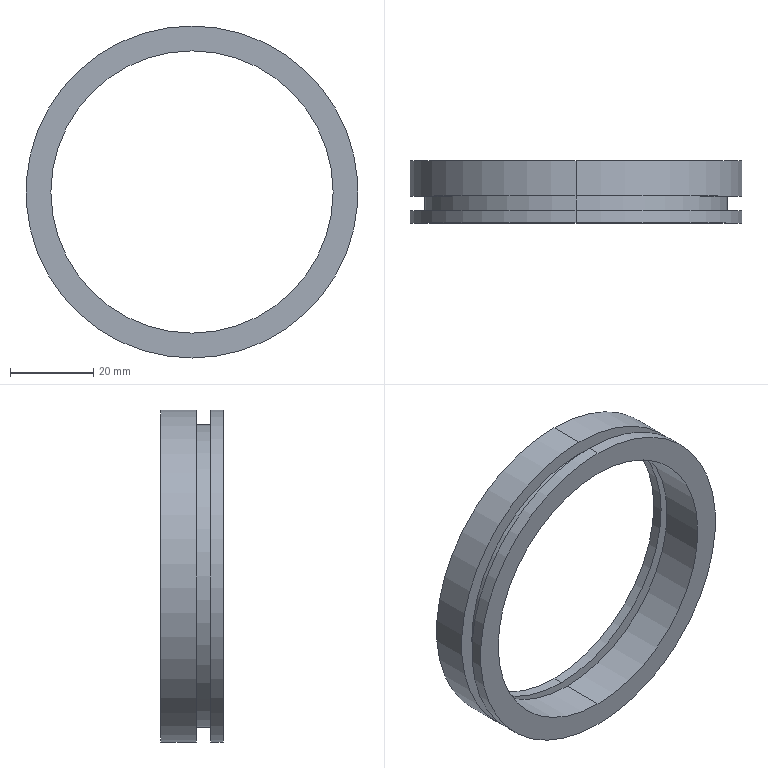Part | SolidWorks | features Revolution 1 | 1 solid | 18 faces | box 80 x 15 x 80 mm | volume 16407 mm3 | cylinder 12 | plane 6 | commonest cylinder face diameters 68 x4 80 x4 73 x2 75 x2
STEP:
#1=CARTESIAN_POINT('',(34.,12.5,37.5));
#2=VERTEX_POINT('',#1);
#3=CARTESIAN_POINT('',(34.,12.5,-37.5));
#4=VERTEX_POINT('',#3);
#5=CARTESIAN_POINT('',(34.,12.5,0.));
#6=DIRECTION('',(0.,-1.,0.));
#7=DIRECTION('',(0.,0.,-1.));
#8=AXIS2_PLACEMENT_3D('',#5,#6,#7);
#9=CIRCLE('',#8,37.5);
#10=EDGE_CURVE('',#2,#4,#9,.T.);
#11=ORIENTED_EDGE('',*,*,#10,.F.);
#12=CARTESIAN_POINT('',(34.,10.5,37.5));
#13=VERTEX_POINT('',#12);
#14=CARTESIAN_POINT('',(34.,0.,37.5));
#15=DIRECTION('',(0.,-1.,0.));
#16=VECTOR('',#15,1000.);
#17=LINE('',#14,#16);
#18=EDGE_CURVE('',#2,#13,#17,.T.);
#19=ORIENTED_EDGE('',*,*,#18,.T.);
#20=CARTESIAN_POINT('',(34.,10.5,-37.5));
#21=VERTEX_POINT('',#20);
#22=CARTESIAN_POINT('',(34.,10.5,0.));
#23=DIRECTION('',(0.,-1.,0.));
#24=DIRECTION('',(0.,0.,-1.));
#25=AXIS2_PLACEMENT_3D('',#22,#23,#24);
#26=CIRCLE('',#25,37.5);
#27=EDGE_CURVE('',#13,#21,#26,.T.);
#28=ORIENTED_EDGE('',*,*,#27,.T.);
#29=CARTESIAN_POINT('',(34.,0.,-37.5));
#30=DIRECTION('',(0.,-1.,0.));
#31=VECTOR('',#30,1000.);
#32=LINE('',#29,#31);
#33=EDGE_CURVE('',#4,#21,#32,.T.);
#34=ORIENTED_EDGE('',*,*,#33,.F.);
#35=EDGE_LOOP('',(#11,#19,#28,#34));
#36=FACE_OUTER_BOUND('',#35,.T.);
#37=CARTESIAN_POINT('',(34.,0.,0.));
#38=DIRECTION('',(0.,-1.,0.));
#39=DIRECTION('',(0.,0.,-1.));
#40=AXIS2_PLACEMENT_3D('',#37,#38,#39);
#41=CYLINDRICAL_SURFACE('',#40,37.5);
#42=ADVANCED_FACE('',(#36),#41,.F.);
#43=CARTESIAN_POINT('',(34.,15.,34.));
#44=VERTEX_POINT('',#43);
#45=CARTESIAN_POINT('',(34.,15.,-34.));
#46=VERTEX_POINT('',#45);
#47=CARTESIAN_POINT('',(34.,15.,0.));
#48=DIRECTION('',(0.,-1.,0.));
#49=DIRECTION('',(0.,0.,-1.));
#50=AXIS2_PLACEMENT_3D('',#47,#48,#49);
#51=CIRCLE('',#50,34.);
#52=EDGE_CURVE('',#44,#46,#51,.T.);
#53=ORIENTED_EDGE('',*,*,#52,.F.);
#54=CARTESIAN_POINT('',(34.,12.5,34.));
#55=VERTEX_POINT('',#54);
#56=CARTESIAN_POINT('',(34.,0.,34.));
#57=DIRECTION('',(0.,-1.,0.));
#58=VECTOR('',#57,1000.);
#59=LINE('',#56,#58);
#60=EDGE_CURVE('',#44,#55,#59,.T.);
#61=ORIENTED_EDGE('',*,*,#60,.T.);
#62=CARTESIAN_POINT('',(34.,12.5,-34.));
#63=VERTEX_POINT('',#62);
#64=CARTESIAN_POINT('',(34.,12.5,0.));
#65=DIRECTION('',(0.,-1.,0.));
#66=DIRECTION('',(0.,0.,-1.));
#67=AXIS2_PLACEMENT_3D('',#64,#65,#66);
#68=CIRCLE('',#67,34.);
#69=EDGE_CURVE('',#55,#63,#68,.T.);
#70=ORIENTED_EDGE('',*,*,#69,.T.);
#71=CARTESIAN_POINT('',(34.,0.,-34.));
#72=DIRECTION('',(0.,-1.,0.));
#73=VECTOR('',#72,1000.);
#74=LINE('',#71,#73);
#75=EDGE_CURVE('',#46,#63,#74,.T.);
#76=ORIENTED_EDGE('',*,*,#75,.F.);
#77=EDGE_LOOP('',(#53,#61,#70,#76));
#78=FACE_OUTER_BOUND('',#77,.T.);
#79=CARTESIAN_POINT('',(34.,0.,0.));
#80=DIRECTION('',(0.,-1.,0.));
#81=DIRECTION('',(0.,0.,-1.));
#82=AXIS2_PLACEMENT_3D('',#79,#80,#81);
#83=CYLINDRICAL_SURFACE('',#82,34.);
#84=ADVANCED_FACE('',(#78),#83,.F.);
#85=CARTESIAN_POINT('',(34.,15.,-40.));
#86=VERTEX_POINT('',#85);
#87=CARTESIAN_POINT('',(34.,15.,40.));
#88=VERTEX_POINT('',#87);
#89=CARTESIAN_POINT('',(34.,15.,0.));
#90=DIRECTION('',(0.,-1.,0.));
#91=DIRECTION('',(0.,0.,-1.));
#92=AXIS2_PLACEMENT_3D('',#89,#90,#91);
#93=CIRCLE('',#92,40.);
#94=EDGE_CURVE('',#86,#88,#93,.T.);
#95=ORIENTED_EDGE('',*,*,#94,.T.);
#96=CARTESIAN_POINT('',(34.,6.5,40.));
#97=VERTEX_POINT('',#96);
#98=CARTESIAN_POINT('',(34.,0.,40.));
#99=DIRECTION('',(0.,-1.,0.));
#100=VECTOR('',#99,1000.);
#101=LINE('',#98,#100);
#102=EDGE_CURVE('',#88,#97,#101,.T.);
#103=ORIENTED_EDGE('',*,*,#102,.T.);
#104=CARTESIAN_POINT('',(34.,6.5,-40.));
#105=VERTEX_POINT('',#104);
#106=CARTESIAN_POINT('',(34.,6.5,0.));
#107=DIRECTION('',(0.,-1.,0.));
#108=DIRECTION('',(0.,0.,-1.));
#109=AXIS2_PLACEMENT_3D('',#106,#107,#108);
#110=CIRCLE('',#109,40.);
#111=EDGE_CURVE('',#105,#97,#110,.T.);
#112=ORIENTED_EDGE('',*,*,#111,.F.);
#113=CARTESIAN_POINT('',(34.,0.,-40.));
#114=DIRECTION('',(0.,-1.,0.));
#115=VECTOR('',#114,1000.);
#116=LINE('',#113,#115);
#117=EDGE_CURVE('',#86,#105,#116,.T.);
#118=ORIENTED_EDGE('',*,*,#117,.F.);
#119=EDGE_LOOP('',(#95,#103,#112,#118));
#120=FACE_OUTER_BOUND('',#119,.T.);
#121=CARTESIAN_POINT('',(34.,0.,0.));
#122=DIRECTION('',(0.,-1.,0.));
#123=DIRECTION('',(0.,0.,-1.));
#124=AXIS2_PLACEMENT_3D('',#121,#122,#123);
#125=CYLINDRICAL_SURFACE('',#124,40.);
#126=ADVANCED_FACE('',(#120),#125,.T.);
#127=CARTESIAN_POINT('',(34.,6.5,-36.5));
#128=VERTEX_POINT('',#127);
#129=CARTESIAN_POINT('',(34.,6.5,36.5));
#130=VERTEX_POINT('',#129);
#131=CARTESIAN_POINT('',(34.,6.5,0.));
#132=DIRECTION('',(0.,-1.,0.));
#133=DIRECTION('',(0.,0.,-1.));
#134=AXIS2_PLACEMENT_3D('',#131,#132,#133);
#135=CIRCLE('',#134,36.5);
#136=EDGE_CURVE('',#128,#130,#135,.T.);
#137=ORIENTED_EDGE('',*,*,#136,.T.);
#138=CARTESIAN_POINT('',(34.,3.,36.5));
#139=VERTEX_POINT('',#138);
#140=CARTESIAN_POINT('',(34.,0.,36.5));
#141=DIRECTION('',(0.,-1.,0.));
#142=VECTOR('',#141,1000.);
#143=LINE('',#140,#142);
#144=EDGE_CURVE('',#130,#139,#143,.T.);
#145=ORIENTED_EDGE('',*,*,#144,.T.);
#146=CARTESIAN_POINT('',(34.,3.,-36.5));
#147=VERTEX_POINT('',#146);
#148=CARTESIAN_POINT('',(34.,3.,0.));
#149=DIRECTION('',(0.,-1.,0.));
#150=DIRECTION('',(0.,0.,-1.));
#151=AXIS2_PLACEMENT_3D('',#148,#149,#150);
#152=CIRCLE('',#151,36.5);
#153=EDGE_CURVE('',#147,#139,#152,.T.);
#154=ORIENTED_EDGE('',*,*,#153,.F.);
#155=CARTESIAN_POINT('',(34.,0.,-36.5));
#156=DIRECTION('',(0.,-1.,0.));
#157=VECTOR('',#156,1000.);
#158=LINE('',#155,#157);
#159=EDGE_CURVE('',#128,#147,#158,.T.);
#160=ORIENTED_EDGE('',*,*,#159,.F.);
#161=EDGE_LOOP('',(#137,#145,#154,#160));
#162=FACE_OUTER_BOUND('',#161,.T.);
#163=CARTESIAN_POINT('',(34.,0.,0.));
#164=DIRECTION('',(0.,-1.,0.));
#165=DIRECTION('',(0.,0.,-1.));
#166=AXIS2_PLACEMENT_3D('',#163,#164,#165);
#167=CYLINDRICAL_SURFACE('',#166,36.5);
#168=ADVANCED_FACE('',(#162),#167,.T.);
#169=CARTESIAN_POINT('',(34.,3.,-40.));
#170=VERTEX_POINT('',#169);
#171=CARTESIAN_POINT('',(34.,3.,40.));
#172=VERTEX_POINT('',#171);
#173=CARTESIAN_POINT('',(34.,3.,0.));
#174=DIRECTION('',(0.,-1.,0.));
#175=DIRECTION('',(0.,0.,-1.));
#176=AXIS2_PLACEMENT_3D('',#173,#174,#175);
#177=CIRCLE('',#176,40.);
#178=EDGE_CURVE('',#170,#172,#177,.T.);
#179=ORIENTED_EDGE('',*,*,#178,.T.);
#180=CARTESIAN_POINT('',(34.,0.,40.));
#181=VERTEX_POINT('',#180);
#182=CARTESIAN_POINT('',(34.,0.,40.));
#183=DIRECTION('',(0.,-1.,0.));
#184=VECTOR('',#183,1000.);
#185=LINE('',#182,#184);
#186=EDGE_CURVE('',#172,#181,#185,.T.);
#187=ORIENTED_EDGE('',*,*,#186,.T.);
#188=CARTESIAN_POINT('',(34.,0.,-40.));
#189=VERTEX_POINT('',#188);
#190=CARTESIAN_POINT('',(34.,0.,0.));
#191=DIRECTION('',(0.,-1.,0.));
#192=DIRECTION('',(0.,0.,-1.));
#193=AXIS2_PLACEMENT_3D('',#190,#191,#192);
#194=CIRCLE('',#193,40.);
#195=EDGE_CURVE('',#189,#181,#194,.T.);
#196=ORIENTED_EDGE('',*,*,#195,.F.);
#197=CARTESIAN_POINT('',(34.,0.,-40.));
#198=DIRECTION('',(0.,-1.,0.));
#199=VECTOR('',#198,1000.);
#200=LINE('',#197,#199);
#201=EDGE_CURVE('',#170,#189,#200,.T.);
#202=ORIENTED_EDGE('',*,*,#201,.F.);
#203=EDGE_LOOP('',(#179,#187,#196,#202));
#204=FACE_OUTER_BOUND('',#203,.T.);
#205=CARTESIAN_POINT('',(34.,0.,0.));
#206=DIRECTION('',(0.,-1.,0.));
#207=DIRECTION('',(0.,0.,-1.));
#208=AXIS2_PLACEMENT_3D('',#205,#206,#207);
#209=CYLINDRICAL_SURFACE('',#208,40.);
#210=ADVANCED_FACE('',(#204),#209,.T.);
#211=CARTESIAN_POINT('',(34.,10.5,34.));
#212=VERTEX_POINT('',#211);
#213=CARTESIAN_POINT('',(34.,10.5,-34.));
#214=VERTEX_POINT('',#213);
#215=CARTESIAN_POINT('',(34.,10.5,0.));
#216=DIRECTION('',(0.,-1.,0.));
#217=DIRECTION('',(0.,0.,-1.));
#218=AXIS2_PLACEMENT_3D('',#215,#216,#217);
#219=CIRCLE('',#218,34.);
#220=EDGE_CURVE('',#212,#214,#219,.T.);
#221=ORIENTED_EDGE('',*,*,#220,.F.);
#222=CARTESIAN_POINT('',(34.,0.,34.));
#223=VERTEX_POINT('',#222);
#224=CARTESIAN_POINT('',(34.,0.,34.));
#225=DIRECTION('',(0.,-1.,0.));
#226=VECTOR('',#225,1000.);
#227=LINE('',#224,#226);
#228=EDGE_CURVE('',#212,#223,#227,.T.);
#229=ORIENTED_EDGE('',*,*,#228,.T.);
#230=CARTESIAN_POINT('',(34.,0.,-34.));
#231=VERTEX_POINT('',#230);
#232=CARTESIAN_POINT('',(34.,0.,0.));
#233=DIRECTION('',(0.,-1.,0.));
#234=DIRECTION('',(0.,0.,-1.));
#235=AXIS2_PLACEMENT_3D('',#232,#233,#234);
#236=CIRCLE('',#235,34.);
#237=EDGE_CURVE('',#223,#231,#236,.T.);
#238=ORIENTED_EDGE('',*,*,#237,.T.);
#239=CARTESIAN_POINT('',(34.,0.,-34.));
#240=DIRECTION('',(0.,-1.,0.));
#241=VECTOR('',#240,1000.);
#242=LINE('',#239,#241);
#243=EDGE_CURVE('',#214,#231,#242,.T.);
#244=ORIENTED_EDGE('',*,*,#243,.F.);
#245=EDGE_LOOP('',(#221,#229,#238,#244));
#246=FACE_OUTER_BOUND('',#245,.T.);
#247=CARTESIAN_POINT('',(34.,0.,0.));
#248=DIRECTION('',(0.,-1.,0.));
#249=DIRECTION('',(0.,0.,-1.));
#250=AXIS2_PLACEMENT_3D('',#247,#248,#249);
#251=CYLINDRICAL_SURFACE('',#250,34.);
#252=ADVANCED_FACE('',(#246),#251,.F.);
#253=ORIENTED_EDGE('',*,*,#228,.F.);
#254=CARTESIAN_POINT('',(34.,10.5,0.));
#255=DIRECTION('',(0.,-1.,0.));
#256=DIRECTION('',(0.,0.,-1.));
#257=AXIS2_PLACEMENT_3D('',#254,#255,#256);
#258=CIRCLE('',#257,34.);
#259=EDGE_CURVE('',#214,#212,#258,.T.);
#260=ORIENTED_EDGE('',*,*,#259,.F.);
#261=ORIENTED_EDGE('',*,*,#243,.T.);
#262=CARTESIAN_POINT('',(34.,0.,0.));
#263=DIRECTION('',(0.,-1.,0.));
#264=DIRECTION('',(0.,0.,-1.));
#265=AXIS2_PLACEMENT_3D('',#262,#263,#264);
#266=CIRCLE('',#265,34.);
#267=EDGE_CURVE('',#231,#223,#266,.T.);
#268=ORIENTED_EDGE('',*,*,#267,.T.);
#269=EDGE_LOOP('',(#253,#260,#261,#268));
#270=FACE_OUTER_BOUND('',#269,.T.);
#271=CARTESIAN_POINT('',(34.,0.,0.));
#272=DIRECTION('',(0.,-1.,0.));
#273=DIRECTION('',(0.,0.,-1.));
#274=AXIS2_PLACEMENT_3D('',#271,#272,#273);
#275=CYLINDRICAL_SURFACE('',#274,34.);
#276=ADVANCED_FACE('',(#270),#275,.F.);
#277=ORIENTED_EDGE('',*,*,#267,.F.);
#278=ORIENTED_EDGE('',*,*,#237,.F.);
#279=EDGE_LOOP('',(#277,#278));
#280=FACE_BOUND('',#279,.T.);
#281=ORIENTED_EDGE('',*,*,#195,.T.);
#282=CARTESIAN_POINT('',(34.,0.,0.));
#283=DIRECTION('',(0.,-1.,0.));
#284=DIRECTION('',(0.,0.,-1.));
#285=AXIS2_PLACEMENT_3D('',#282,#283,#284);
#286=CIRCLE('',#285,40.);
#287=EDGE_CURVE('',#181,#189,#286,.T.);
#288=ORIENTED_EDGE('',*,*,#287,.T.);
#289=EDGE_LOOP('',(#281,#288));
#290=FACE_OUTER_BOUND('',#289,.T.);
#291=CARTESIAN_POINT('',(0.,0.,0.));
#292=DIRECTION('',(0.,1.,0.));
#293=DIRECTION('',(0.,0.,1.));
#294=AXIS2_PLACEMENT_3D('',#291,#292,#293);
#295=PLANE('',#294);
#296=ADVANCED_FACE('',(#280,#290),#295,.F.);
#297=ORIENTED_EDGE('',*,*,#186,.F.);
#298=CARTESIAN_POINT('',(34.,3.,0.));
#299=DIRECTION('',(0.,-1.,0.));
#300=DIRECTION('',(0.,0.,-1.));
#301=AXIS2_PLACEMENT_3D('',#298,#299,#300);
#302=CIRCLE('',#301,40.);
#303=EDGE_CURVE('',#172,#170,#302,.T.);
#304=ORIENTED_EDGE('',*,*,#303,.T.);
#305=ORIENTED_EDGE('',*,*,#201,.T.);
#306=ORIENTED_EDGE('',*,*,#287,.F.);
#307=EDGE_LOOP('',(#297,#304,#305,#306));
#308=FACE_OUTER_BOUND('',#307,.T.);
#309=CARTESIAN_POINT('',(34.,0.,0.));
#310=DIRECTION('',(0.,-1.,0.));
#311=DIRECTION('',(0.,0.,-1.));
#312=AXIS2_PLACEMENT_3D('',#309,#310,#311);
#313=CYLINDRICAL_SURFACE('',#312,40.);
#314=ADVANCED_FACE('',(#308),#313,.T.);
#315=ORIENTED_EDGE('',*,*,#178,.F.);
#316=ORIENTED_EDGE('',*,*,#303,.F.);
#317=EDGE_LOOP('',(#315,#316));
#318=FACE_OUTER_BOUND('',#317,.T.);
#319=ORIENTED_EDGE('',*,*,#153,.T.);
#320=CARTESIAN_POINT('',(34.,3.,0.));
#321=DIRECTION('',(0.,-1.,0.));
#322=DIRECTION('',(0.,0.,-1.));
#323=AXIS2_PLACEMENT_3D('',#320,#321,#322);
#324=CIRCLE('',#323,36.5);
#325=EDGE_CURVE('',#139,#147,#324,.T.);
#326=ORIENTED_EDGE('',*,*,#325,.T.);
#327=EDGE_LOOP('',(#319,#326));
#328=FACE_BOUND('',#327,.T.);
#329=CARTESIAN_POINT('',(-2.5,3.,0.));
#330=DIRECTION('',(0.,-1.,0.));
#331=DIRECTION('',(0.,0.,-1.));
#332=AXIS2_PLACEMENT_3D('',#329,#330,#331);
#333=PLANE('',#332);
#334=ADVANCED_FACE('',(#318,#328),#333,.F.);
#335=ORIENTED_EDGE('',*,*,#144,.F.);
#336=CARTESIAN_POINT('',(34.,6.5,0.));
#337=DIRECTION('',(0.,-1.,0.));
#338=DIRECTION('',(0.,0.,-1.));
#339=AXIS2_PLACEMENT_3D('',#336,#337,#338);
#340=CIRCLE('',#339,36.5);
#341=EDGE_CURVE('',#130,#128,#340,.T.);
#342=ORIENTED_EDGE('',*,*,#341,.T.);
#343=ORIENTED_EDGE('',*,*,#159,.T.);
#344=ORIENTED_EDGE('',*,*,#325,.F.);
#345=EDGE_LOOP('',(#335,#342,#343,#344));
#346=FACE_OUTER_BOUND('',#345,.T.);
#347=CARTESIAN_POINT('',(34.,0.,0.));
#348=DIRECTION('',(0.,-1.,0.));
#349=DIRECTION('',(0.,0.,-1.));
#350=AXIS2_PLACEMENT_3D('',#347,#348,#349);
#351=CYLINDRICAL_SURFACE('',#350,36.5);
#352=ADVANCED_FACE('',(#346),#351,.T.);
#353=ORIENTED_EDGE('',*,*,#136,.F.);
#354=ORIENTED_EDGE('',*,*,#341,.F.);
#355=EDGE_LOOP('',(#353,#354));
#356=FACE_BOUND('',#355,.T.);
#357=ORIENTED_EDGE('',*,*,#111,.T.);
#358=CARTESIAN_POINT('',(34.,6.5,0.));
#359=DIRECTION('',(0.,-1.,0.));
#360=DIRECTION('',(0.,0.,-1.));
#361=AXIS2_PLACEMENT_3D('',#358,#359,#360);
#362=CIRCLE('',#361,40.);
#363=EDGE_CURVE('',#97,#105,#362,.T.);
#364=ORIENTED_EDGE('',*,*,#363,.T.);
#365=EDGE_LOOP('',(#357,#364));
#366=FACE_OUTER_BOUND('',#365,.T.);
#367=CARTESIAN_POINT('',(-6.,6.5,0.));
#368=DIRECTION('',(0.,1.,0.));
#369=DIRECTION('',(0.,0.,1.));
#370=AXIS2_PLACEMENT_3D('',#367,#368,#369);
#371=PLANE('',#370);
#372=ADVANCED_FACE('',(#356,#366),#371,.F.);
#373=ORIENTED_EDGE('',*,*,#102,.F.);
#374=CARTESIAN_POINT('',(34.,15.,0.));
#375=DIRECTION('',(0.,-1.,0.));
#376=DIRECTION('',(0.,0.,-1.));
#377=AXIS2_PLACEMENT_3D('',#374,#375,#376);
#378=CIRCLE('',#377,40.);
#379=EDGE_CURVE('',#88,#86,#378,.T.);
#380=ORIENTED_EDGE('',*,*,#379,.T.);
#381=ORIENTED_EDGE('',*,*,#117,.T.);
#382=ORIENTED_EDGE('',*,*,#363,.F.);
#383=EDGE_LOOP('',(#373,#380,#381,#382));
#384=FACE_OUTER_BOUND('',#383,.T.);
#385=CARTESIAN_POINT('',(34.,0.,0.));
#386=DIRECTION('',(0.,-1.,0.));
#387=DIRECTION('',(0.,0.,-1.));
#388=AXIS2_PLACEMENT_3D('',#385,#386,#387);
#389=CYLINDRICAL_SURFACE('',#388,40.);
#390=ADVANCED_FACE('',(#384),#389,.T.);
#391=ORIENTED_EDGE('',*,*,#94,.F.);
#392=ORIENTED_EDGE('',*,*,#379,.F.);
#393=EDGE_LOOP('',(#391,#392));
#394=FACE_OUTER_BOUND('',#393,.T.);
#395=CARTESIAN_POINT('',(34.,15.,0.));
#396=DIRECTION('',(0.,-1.,0.));
#397=DIRECTION('',(0.,0.,-1.));
#398=AXIS2_PLACEMENT_3D('',#395,#396,#397);
#399=CIRCLE('',#398,34.);
#400=EDGE_CURVE('',#46,#44,#399,.T.);
#401=ORIENTED_EDGE('',*,*,#400,.T.);
#402=ORIENTED_EDGE('',*,*,#52,.T.);
#403=EDGE_LOOP('',(#401,#402));
#404=FACE_BOUND('',#403,.T.);
#405=CARTESIAN_POINT('',(0.,15.,0.));
#406=DIRECTION('',(0.,-1.,0.));
#407=DIRECTION('',(0.,0.,-1.));
#408=AXIS2_PLACEMENT_3D('',#405,#406,#407);
#409=PLANE('',#408);
#410=ADVANCED_FACE('',(#394,#404),#409,.F.);
#411=ORIENTED_EDGE('',*,*,#60,.F.);
#412=ORIENTED_EDGE('',*,*,#400,.F.);
#413=ORIENTED_EDGE('',*,*,#75,.T.);
#414=CARTESIAN_POINT('',(34.,12.5,0.));
#415=DIRECTION('',(0.,-1.,0.));
#416=DIRECTION('',(0.,0.,-1.));
#417=AXIS2_PLACEMENT_3D('',#414,#415,#416);
#418=CIRCLE('',#417,34.);
#419=EDGE_CURVE('',#63,#55,#418,.T.);
#420=ORIENTED_EDGE('',*,*,#419,.T.);
#421=EDGE_LOOP('',(#411,#412,#413,#420));
#422=FACE_OUTER_BOUND('',#421,.T.);
#423=CARTESIAN_POINT('',(34.,0.,0.));
#424=DIRECTION('',(0.,-1.,0.));
#425=DIRECTION('',(0.,0.,-1.));
#426=AXIS2_PLACEMENT_3D('',#423,#424,#425);
#427=CYLINDRICAL_SURFACE('',#426,34.);
#428=ADVANCED_FACE('',(#422),#427,.F.);
#429=ORIENTED_EDGE('',*,*,#419,.F.);
#430=ORIENTED_EDGE('',*,*,#69,.F.);
#431=EDGE_LOOP('',(#429,#430));
#432=FACE_BOUND('',#431,.T.);
#433=CARTESIAN_POINT('',(34.,12.5,0.));
#434=DIRECTION('',(0.,-1.,0.));
#435=DIRECTION('',(0.,0.,-1.));
#436=AXIS2_PLACEMENT_3D('',#433,#434,#435);
#437=CIRCLE('',#436,37.5);
#438=EDGE_CURVE('',#4,#2,#437,.T.);
#439=ORIENTED_EDGE('',*,*,#438,.T.);
#440=ORIENTED_EDGE('',*,*,#10,.T.);
#441=EDGE_LOOP('',(#439,#440));
#442=FACE_OUTER_BOUND('',#441,.T.);
#443=CARTESIAN_POINT('',(0.,12.5,0.));
#444=DIRECTION('',(0.,1.,0.));
#445=DIRECTION('',(0.,0.,1.));
#446=AXIS2_PLACEMENT_3D('',#443,#444,#445);
#447=PLANE('',#446);
#448=ADVANCED_FACE('',(#432,#442),#447,.F.);
#449=ORIENTED_EDGE('',*,*,#18,.F.);
#450=ORIENTED_EDGE('',*,*,#438,.F.);
#451=ORIENTED_EDGE('',*,*,#33,.T.);
#452=CARTESIAN_POINT('',(34.,10.5,0.));
#453=DIRECTION('',(0.,-1.,0.));
#454=DIRECTION('',(0.,0.,-1.));
#455=AXIS2_PLACEMENT_3D('',#452,#453,#454);
#456=CIRCLE('',#455,37.5);
#457=EDGE_CURVE('',#21,#13,#456,.T.);
#458=ORIENTED_EDGE('',*,*,#457,.T.);
#459=EDGE_LOOP('',(#449,#450,#451,#458));
#460=FACE_OUTER_BOUND('',#459,.T.);
#461=CARTESIAN_POINT('',(34.,0.,0.));
#462=DIRECTION('',(0.,-1.,0.));
#463=DIRECTION('',(0.,0.,-1.));
#464=AXIS2_PLACEMENT_3D('',#461,#462,#463);
#465=CYLINDRICAL_SURFACE('',#464,37.5);
#466=ADVANCED_FACE('',(#460),#465,.F.);
#467=ORIENTED_EDGE('',*,*,#457,.F.);
#468=ORIENTED_EDGE('',*,*,#27,.F.);
#469=EDGE_LOOP('',(#467,#468));
#470=FACE_OUTER_BOUND('',#469,.T.);
#471=ORIENTED_EDGE('',*,*,#259,.T.);
#472=ORIENTED_EDGE('',*,*,#220,.T.);
#473=EDGE_LOOP('',(#471,#472));
#474=FACE_BOUND('',#473,.T.);
#475=CARTESIAN_POINT('',(-3.5,10.5,0.));
#476=DIRECTION('',(0.,-1.,0.));
#477=DIRECTION('',(0.,0.,-1.));
#478=AXIS2_PLACEMENT_3D('',#475,#476,#477);
#479=PLANE('',#478);
#480=ADVANCED_FACE('',(#470,#474),#479,.F.);
#481=CLOSED_SHELL('',(#42,#84,#126,#168,#210,#252,#276,#296,#314,#334,#352,#372,#390,#410,#428,#448,#466,#480));
#482=MANIFOLD_SOLID_BREP('',#481);
#483=CARTESIAN_POINT('',(0.,0.,0.));
#484=DIRECTION('',(0.,0.,1.));
#485=DIRECTION('',(1.,0.,0.));
#486=AXIS2_PLACEMENT_3D('',#483,#484,#485);
#487=(LENGTH_UNIT()NAMED_UNIT(*)SI_UNIT(.MILLI.,.METRE.));
#488=UNCERTAINTY_MEASURE_WITH_UNIT(LENGTH_MEASURE(0.00001),#487,'','');
#489=(NAMED_UNIT(*)PLANE_ANGLE_UNIT()SI_UNIT($,.RADIAN.));
#490=(NAMED_UNIT(*)SI_UNIT($,.STERADIAN.)SOLID_ANGLE_UNIT());
#491=(GEOMETRIC_REPRESENTATION_CONTEXT(3)GLOBAL_UNCERTAINTY_ASSIGNED_CONTEXT((#488))GLOBAL_UNIT_ASSIGNED_CONTEXT((#487,#489,#490))REPRESENTATION_CONTEXT('',''));
#492=ADVANCED_BREP_SHAPE_REPRESENTATION('',(#482,#486),#491);